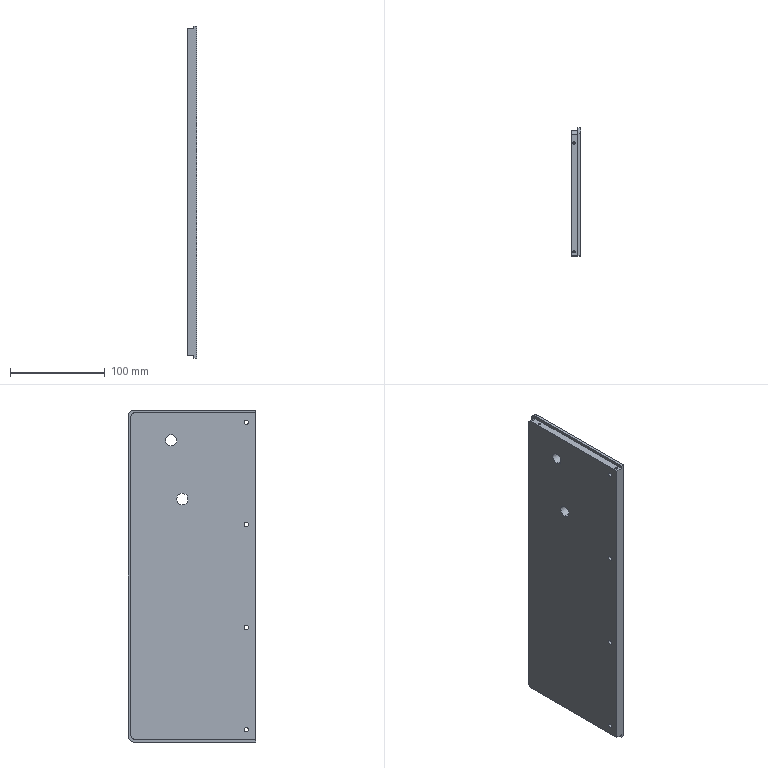Part | SolidWorks | features Cut 44, HoleWzd 41, MoveFace 38, ICE 28, DelFace 17, Fillet 17, MirrorPattern 3, SweepCut 2, Extrusion 1 | 1 solid | 78 faces | box 10 x 135 x 351 mm | volume 457423 mm3 | cylinder 38 | cone 30 | plane 10 | commonest cylinder face diameters 2.5 x22 4.5 x8 12 x6 8 x2